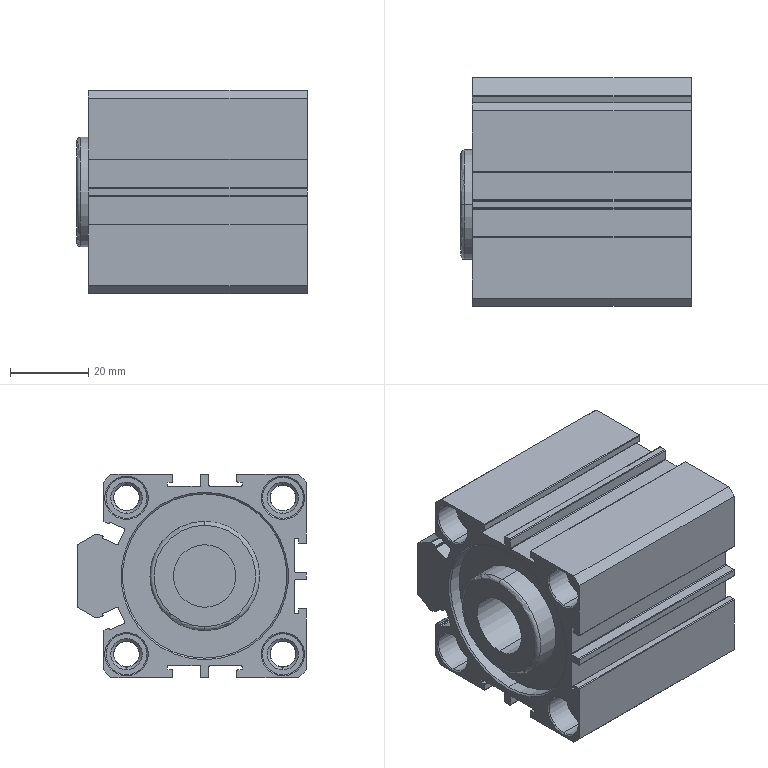Part | SolidWorks | features MBimport 1 | 1 solid | 255 faces | box 59 x 58.5 x 52 mm | volume 79787 mm3 | cylinder 110 | plane 87 | cone 56 | torus 2 | commonest cylinder face diameters 0.4 x46 6.647 x16 10.5 x16 0.8 x10 6.5 x8 8.566 x4